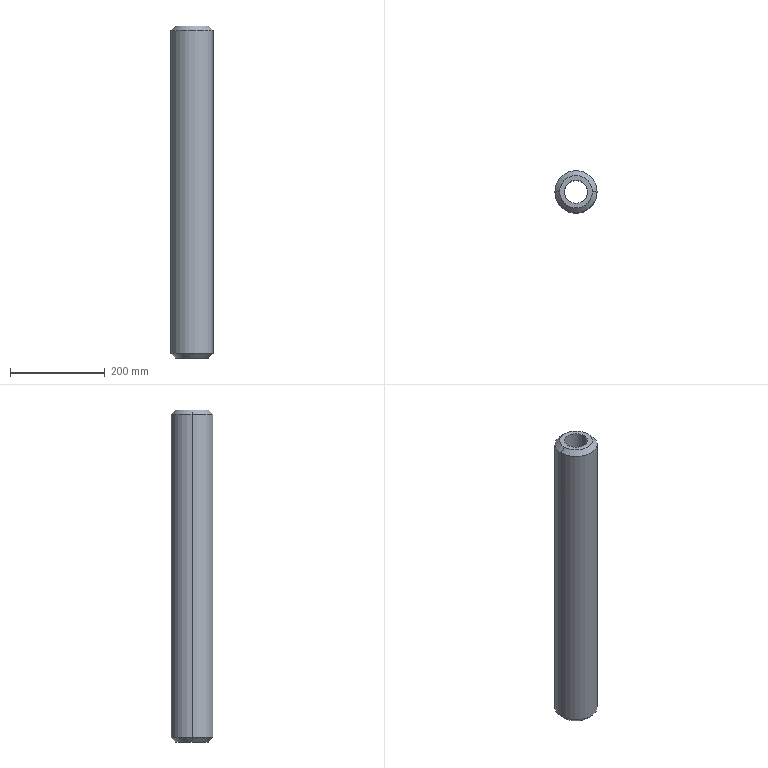Part | SolidWorks | features Chamfer 1, ExtruThin 1 | 1 solid | 10 faces | box 89 x 89 x 700 mm | volume 3008913 mm3 | cone 4 | cylinder 4 | plane 2 | commonest cylinder face diameters 49 x2 89 x2
STEP:
#1=CARTESIAN_POINT('',(-34.5,0.,-350.));
#2=VERTEX_POINT('',#1);
#3=CARTESIAN_POINT('',(34.5,0.,-350.));
#4=VERTEX_POINT('',#3);
#5=CARTESIAN_POINT('',(0.,0.,-350.));
#6=DIRECTION('',(0.,0.,-1.));
#7=DIRECTION('',(1.,0.,0.));
#8=AXIS2_PLACEMENT_3D('',#5,#6,#7);
#9=CIRCLE('',#8,34.5);
#10=EDGE_CURVE('',#2,#4,#9,.T.);
#11=ORIENTED_EDGE('',*,*,#10,.F.);
#12=CARTESIAN_POINT('',(-44.5,0.,-340.));
#13=VERTEX_POINT('',#12);
#14=CARTESIAN_POINT('',(-44.5,0.,-340.));
#15=DIRECTION('',(-0.7071,0.,0.7071));
#16=VECTOR('',#15,1000.);
#17=LINE('',#14,#16);
#18=EDGE_CURVE('',#2,#13,#17,.T.);
#19=ORIENTED_EDGE('',*,*,#18,.T.);
#20=CARTESIAN_POINT('',(44.5,0.,-340.));
#21=VERTEX_POINT('',#20);
#22=CARTESIAN_POINT('',(0.,0.,-340.));
#23=DIRECTION('',(0.,0.,1.));
#24=DIRECTION('',(1.,0.,0.));
#25=AXIS2_PLACEMENT_3D('',#22,#23,#24);
#26=CIRCLE('',#25,44.5);
#27=EDGE_CURVE('',#21,#13,#26,.T.);
#28=ORIENTED_EDGE('',*,*,#27,.F.);
#29=CARTESIAN_POINT('',(44.5,0.,-340.));
#30=DIRECTION('',(0.7071,0.,0.7071));
#31=VECTOR('',#30,1000.);
#32=LINE('',#29,#31);
#33=EDGE_CURVE('',#4,#21,#32,.T.);
#34=ORIENTED_EDGE('',*,*,#33,.F.);
#35=EDGE_LOOP('',(#11,#19,#28,#34));
#36=FACE_OUTER_BOUND('',#35,.T.);
#37=CARTESIAN_POINT('',(0.,0.,-340.));
#38=DIRECTION('',(0.,0.,1.));
#39=DIRECTION('',(1.,0.,0.));
#40=AXIS2_PLACEMENT_3D('',#37,#38,#39);
#41=CONICAL_SURFACE('',#40,44.5,0.7854);
#42=ADVANCED_FACE('',(#36),#41,.T.);
#43=CARTESIAN_POINT('',(34.5,0.,350.));
#44=VERTEX_POINT('',#43);
#45=CARTESIAN_POINT('',(-34.5,0.,350.));
#46=VERTEX_POINT('',#45);
#47=CARTESIAN_POINT('',(0.,0.,350.));
#48=DIRECTION('',(0.,0.,1.));
#49=DIRECTION('',(1.,0.,0.));
#50=AXIS2_PLACEMENT_3D('',#47,#48,#49);
#51=CIRCLE('',#50,34.5);
#52=EDGE_CURVE('',#44,#46,#51,.T.);
#53=ORIENTED_EDGE('',*,*,#52,.F.);
#54=CARTESIAN_POINT('',(44.5,0.,340.));
#55=VERTEX_POINT('',#54);
#56=CARTESIAN_POINT('',(34.5,0.,350.));
#57=DIRECTION('',(0.7071,0.,-0.7071));
#58=VECTOR('',#57,1000.);
#59=LINE('',#56,#58);
#60=EDGE_CURVE('',#44,#55,#59,.T.);
#61=ORIENTED_EDGE('',*,*,#60,.T.);
#62=CARTESIAN_POINT('',(-44.5,0.,340.));
#63=VERTEX_POINT('',#62);
#64=CARTESIAN_POINT('',(0.,0.,340.));
#65=DIRECTION('',(0.,0.,-1.));
#66=DIRECTION('',(1.,0.,0.));
#67=AXIS2_PLACEMENT_3D('',#64,#65,#66);
#68=CIRCLE('',#67,44.5);
#69=EDGE_CURVE('',#63,#55,#68,.T.);
#70=ORIENTED_EDGE('',*,*,#69,.F.);
#71=CARTESIAN_POINT('',(-34.5,0.,350.));
#72=DIRECTION('',(-0.7071,0.,-0.7071));
#73=VECTOR('',#72,1000.);
#74=LINE('',#71,#73);
#75=EDGE_CURVE('',#46,#63,#74,.T.);
#76=ORIENTED_EDGE('',*,*,#75,.F.);
#77=EDGE_LOOP('',(#53,#61,#70,#76));
#78=FACE_OUTER_BOUND('',#77,.T.);
#79=CARTESIAN_POINT('',(0.,0.,350.));
#80=DIRECTION('',(0.,0.,-1.));
#81=DIRECTION('',(-1.,0.,0.));
#82=AXIS2_PLACEMENT_3D('',#79,#80,#81);
#83=CONICAL_SURFACE('',#82,34.5,0.7854);
#84=ADVANCED_FACE('',(#78),#83,.T.);
#85=CARTESIAN_POINT('',(-24.5,0.,350.));
#86=VERTEX_POINT('',#85);
#87=CARTESIAN_POINT('',(24.5,0.,350.));
#88=VERTEX_POINT('',#87);
#89=CARTESIAN_POINT('',(0.,0.,350.));
#90=DIRECTION('',(0.,0.,1.));
#91=DIRECTION('',(1.,0.,0.));
#92=AXIS2_PLACEMENT_3D('',#89,#90,#91);
#93=CIRCLE('',#92,24.5);
#94=EDGE_CURVE('',#86,#88,#93,.T.);
#95=ORIENTED_EDGE('',*,*,#94,.T.);
#96=CARTESIAN_POINT('',(24.5,0.,-350.));
#97=VERTEX_POINT('',#96);
#98=CARTESIAN_POINT('',(24.5,0.,350.));
#99=DIRECTION('',(0.,0.,-1.));
#100=VECTOR('',#99,1000.);
#101=LINE('',#98,#100);
#102=EDGE_CURVE('',#88,#97,#101,.T.);
#103=ORIENTED_EDGE('',*,*,#102,.T.);
#104=CARTESIAN_POINT('',(-24.5,0.,-350.));
#105=VERTEX_POINT('',#104);
#106=CARTESIAN_POINT('',(0.,0.,-350.));
#107=DIRECTION('',(0.,0.,1.));
#108=DIRECTION('',(1.,0.,0.));
#109=AXIS2_PLACEMENT_3D('',#106,#107,#108);
#110=CIRCLE('',#109,24.5);
#111=EDGE_CURVE('',#105,#97,#110,.T.);
#112=ORIENTED_EDGE('',*,*,#111,.F.);
#113=CARTESIAN_POINT('',(-24.5,0.,350.));
#114=DIRECTION('',(0.,0.,-1.));
#115=VECTOR('',#114,1000.);
#116=LINE('',#113,#115);
#117=EDGE_CURVE('',#86,#105,#116,.T.);
#118=ORIENTED_EDGE('',*,*,#117,.F.);
#119=EDGE_LOOP('',(#95,#103,#112,#118));
#120=FACE_OUTER_BOUND('',#119,.T.);
#121=CARTESIAN_POINT('',(0.,0.,350.));
#122=DIRECTION('',(0.,0.,-1.));
#123=DIRECTION('',(-1.,0.,0.));
#124=AXIS2_PLACEMENT_3D('',#121,#122,#123);
#125=CYLINDRICAL_SURFACE('',#124,24.5);
#126=ADVANCED_FACE('',(#120),#125,.F.);
#127=ORIENTED_EDGE('',*,*,#69,.T.);
#128=CARTESIAN_POINT('',(44.5,0.,350.));
#129=DIRECTION('',(0.,0.,-1.));
#130=VECTOR('',#129,1000.);
#131=LINE('',#128,#130);
#132=EDGE_CURVE('',#55,#21,#131,.T.);
#133=ORIENTED_EDGE('',*,*,#132,.T.);
#134=ORIENTED_EDGE('',*,*,#27,.T.);
#135=CARTESIAN_POINT('',(-44.5,0.,350.));
#136=DIRECTION('',(0.,0.,-1.));
#137=VECTOR('',#136,1000.);
#138=LINE('',#135,#137);
#139=EDGE_CURVE('',#63,#13,#138,.T.);
#140=ORIENTED_EDGE('',*,*,#139,.F.);
#141=EDGE_LOOP('',(#127,#133,#134,#140));
#142=FACE_OUTER_BOUND('',#141,.T.);
#143=CARTESIAN_POINT('',(0.,0.,350.));
#144=DIRECTION('',(0.,0.,-1.));
#145=DIRECTION('',(-1.,0.,0.));
#146=AXIS2_PLACEMENT_3D('',#143,#144,#145);
#147=CYLINDRICAL_SURFACE('',#146,44.5);
#148=ADVANCED_FACE('',(#142),#147,.T.);
#149=CARTESIAN_POINT('',(0.,0.,350.));
#150=DIRECTION('',(0.,0.,1.));
#151=DIRECTION('',(1.,0.,0.));
#152=AXIS2_PLACEMENT_3D('',#149,#150,#151);
#153=CIRCLE('',#152,34.5);
#154=EDGE_CURVE('',#46,#44,#153,.T.);
#155=ORIENTED_EDGE('',*,*,#154,.T.);
#156=ORIENTED_EDGE('',*,*,#52,.T.);
#157=EDGE_LOOP('',(#155,#156));
#158=FACE_OUTER_BOUND('',#157,.T.);
#159=ORIENTED_EDGE('',*,*,#94,.F.);
#160=CARTESIAN_POINT('',(0.,0.,350.));
#161=DIRECTION('',(0.,0.,1.));
#162=DIRECTION('',(1.,0.,0.));
#163=AXIS2_PLACEMENT_3D('',#160,#161,#162);
#164=CIRCLE('',#163,24.5);
#165=EDGE_CURVE('',#88,#86,#164,.T.);
#166=ORIENTED_EDGE('',*,*,#165,.F.);
#167=EDGE_LOOP('',(#159,#166));
#168=FACE_BOUND('',#167,.T.);
#169=CARTESIAN_POINT('',(0.,0.,350.));
#170=DIRECTION('',(0.,0.,1.));
#171=DIRECTION('',(1.,0.,0.));
#172=AXIS2_PLACEMENT_3D('',#169,#170,#171);
#173=PLANE('',#172);
#174=ADVANCED_FACE('',(#158,#168),#173,.T.);
#175=CARTESIAN_POINT('',(0.,0.,-350.));
#176=DIRECTION('',(0.,0.,-1.));
#177=DIRECTION('',(1.,0.,0.));
#178=AXIS2_PLACEMENT_3D('',#175,#176,#177);
#179=CIRCLE('',#178,34.5);
#180=EDGE_CURVE('',#4,#2,#179,.T.);
#181=ORIENTED_EDGE('',*,*,#180,.T.);
#182=ORIENTED_EDGE('',*,*,#10,.T.);
#183=EDGE_LOOP('',(#181,#182));
#184=FACE_OUTER_BOUND('',#183,.T.);
#185=ORIENTED_EDGE('',*,*,#111,.T.);
#186=CARTESIAN_POINT('',(0.,0.,-350.));
#187=DIRECTION('',(0.,0.,1.));
#188=DIRECTION('',(1.,0.,0.));
#189=AXIS2_PLACEMENT_3D('',#186,#187,#188);
#190=CIRCLE('',#189,24.5);
#191=EDGE_CURVE('',#97,#105,#190,.T.);
#192=ORIENTED_EDGE('',*,*,#191,.T.);
#193=EDGE_LOOP('',(#185,#192));
#194=FACE_BOUND('',#193,.T.);
#195=CARTESIAN_POINT('',(0.,0.,-350.));
#196=DIRECTION('',(0.,0.,1.));
#197=DIRECTION('',(1.,0.,0.));
#198=AXIS2_PLACEMENT_3D('',#195,#196,#197);
#199=PLANE('',#198);
#200=ADVANCED_FACE('',(#184,#194),#199,.F.);
#201=ORIENTED_EDGE('',*,*,#132,.F.);
#202=CARTESIAN_POINT('',(0.,0.,340.));
#203=DIRECTION('',(0.,0.,-1.));
#204=DIRECTION('',(1.,0.,0.));
#205=AXIS2_PLACEMENT_3D('',#202,#203,#204);
#206=CIRCLE('',#205,44.5);
#207=EDGE_CURVE('',#55,#63,#206,.T.);
#208=ORIENTED_EDGE('',*,*,#207,.T.);
#209=ORIENTED_EDGE('',*,*,#139,.T.);
#210=CARTESIAN_POINT('',(0.,0.,-340.));
#211=DIRECTION('',(0.,0.,1.));
#212=DIRECTION('',(1.,0.,0.));
#213=AXIS2_PLACEMENT_3D('',#210,#211,#212);
#214=CIRCLE('',#213,44.5);
#215=EDGE_CURVE('',#13,#21,#214,.T.);
#216=ORIENTED_EDGE('',*,*,#215,.T.);
#217=EDGE_LOOP('',(#201,#208,#209,#216));
#218=FACE_OUTER_BOUND('',#217,.T.);
#219=CARTESIAN_POINT('',(0.,0.,350.));
#220=DIRECTION('',(0.,0.,-1.));
#221=DIRECTION('',(-1.,0.,0.));
#222=AXIS2_PLACEMENT_3D('',#219,#220,#221);
#223=CYLINDRICAL_SURFACE('',#222,44.5);
#224=ADVANCED_FACE('',(#218),#223,.T.);
#225=ORIENTED_EDGE('',*,*,#102,.F.);
#226=ORIENTED_EDGE('',*,*,#165,.T.);
#227=ORIENTED_EDGE('',*,*,#117,.T.);
#228=ORIENTED_EDGE('',*,*,#191,.F.);
#229=EDGE_LOOP('',(#225,#226,#227,#228));
#230=FACE_OUTER_BOUND('',#229,.T.);
#231=CARTESIAN_POINT('',(0.,0.,350.));
#232=DIRECTION('',(0.,0.,-1.));
#233=DIRECTION('',(-1.,0.,0.));
#234=AXIS2_PLACEMENT_3D('',#231,#232,#233);
#235=CYLINDRICAL_SURFACE('',#234,24.5);
#236=ADVANCED_FACE('',(#230),#235,.F.);
#237=ORIENTED_EDGE('',*,*,#60,.F.);
#238=ORIENTED_EDGE('',*,*,#154,.F.);
#239=ORIENTED_EDGE('',*,*,#75,.T.);
#240=ORIENTED_EDGE('',*,*,#207,.F.);
#241=EDGE_LOOP('',(#237,#238,#239,#240));
#242=FACE_OUTER_BOUND('',#241,.T.);
#243=CARTESIAN_POINT('',(0.,0.,350.));
#244=DIRECTION('',(0.,0.,-1.));
#245=DIRECTION('',(-1.,0.,0.));
#246=AXIS2_PLACEMENT_3D('',#243,#244,#245);
#247=CONICAL_SURFACE('',#246,34.5,0.7854);
#248=ADVANCED_FACE('',(#242),#247,.T.);
#249=ORIENTED_EDGE('',*,*,#18,.F.);
#250=ORIENTED_EDGE('',*,*,#180,.F.);
#251=ORIENTED_EDGE('',*,*,#33,.T.);
#252=ORIENTED_EDGE('',*,*,#215,.F.);
#253=EDGE_LOOP('',(#249,#250,#251,#252));
#254=FACE_OUTER_BOUND('',#253,.T.);
#255=CARTESIAN_POINT('',(0.,0.,-340.));
#256=DIRECTION('',(0.,0.,1.));
#257=DIRECTION('',(1.,0.,0.));
#258=AXIS2_PLACEMENT_3D('',#255,#256,#257);
#259=CONICAL_SURFACE('',#258,44.5,0.7854);
#260=ADVANCED_FACE('',(#254),#259,.T.);
#261=CLOSED_SHELL('',(#42,#84,#126,#148,#174,#200,#224,#236,#248,#260));
#262=MANIFOLD_SOLID_BREP('',#261);
#263=CARTESIAN_POINT('',(0.,0.,0.));
#264=DIRECTION('',(0.,0.,1.));
#265=DIRECTION('',(1.,0.,0.));
#266=AXIS2_PLACEMENT_3D('',#263,#264,#265);
#267=(LENGTH_UNIT()NAMED_UNIT(*)SI_UNIT(.MILLI.,.METRE.));
#268=UNCERTAINTY_MEASURE_WITH_UNIT(LENGTH_MEASURE(0.00001),#267,'','');
#269=(NAMED_UNIT(*)PLANE_ANGLE_UNIT()SI_UNIT($,.RADIAN.));
#270=(NAMED_UNIT(*)SI_UNIT($,.STERADIAN.)SOLID_ANGLE_UNIT());
#271=(GEOMETRIC_REPRESENTATION_CONTEXT(3)GLOBAL_UNCERTAINTY_ASSIGNED_CONTEXT((#268))GLOBAL_UNIT_ASSIGNED_CONTEXT((#267,#269,#270))REPRESENTATION_CONTEXT('',''));
#272=ADVANCED_BREP_SHAPE_REPRESENTATION('',(#262,#266),#271);